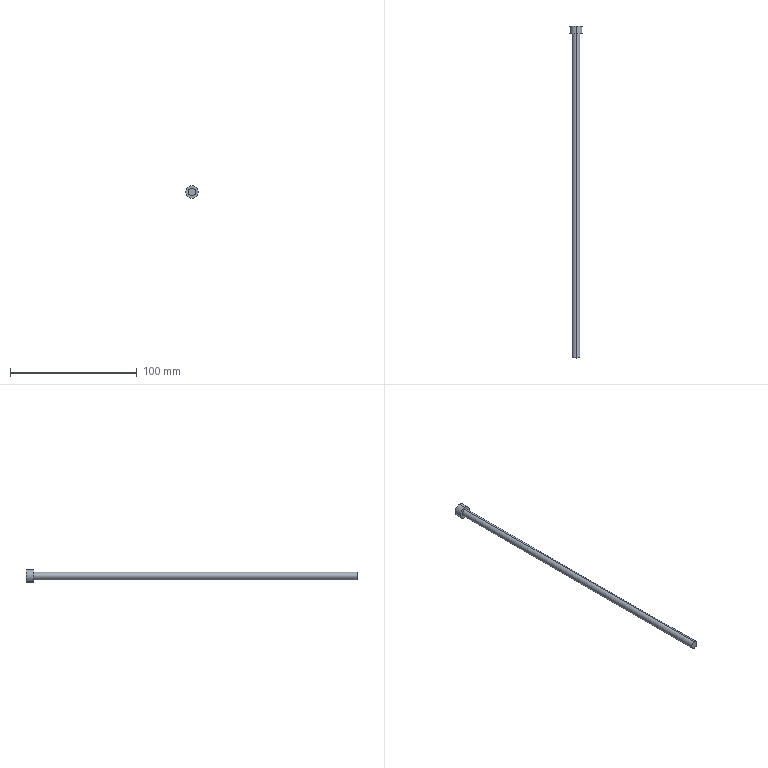Part | STEP file | 1 solid | 7 faces | box 10 x 262.36 x 10 mm | volume 7720 mm3 | cylinder 4 | plane 3 | commonest cylinder face diameters 6 x2 10 x2
STEP:
#1=CARTESIAN_POINT('',(0.,0.,0.));
#2=DIRECTION('',(0.,0.,1.));
#3=DIRECTION('',(1.,0.,0.));
#4=AXIS2_PLACEMENT_3D('',#1,#2,#3);
#5=CARTESIAN_POINT('',(-135.864,290.5,51.072));
#6=VERTEX_POINT('',#5);
#7=CARTESIAN_POINT('',(-135.864,290.5,61.072));
#8=VERTEX_POINT('',#7);
#9=CARTESIAN_POINT('',(-135.864,290.5,56.072));
#10=DIRECTION('',(0.,-1.,0.));
#11=DIRECTION('',(0.,0.,-1.));
#12=AXIS2_PLACEMENT_3D('',#9,#10,#11);
#13=CIRCLE('',#12,5.);
#14=CARTESIAN_POINT('',(-135.864,290.5,56.072));
#15=DIRECTION('',(0.,-1.,0.));
#16=DIRECTION('',(0.,0.,-1.));
#17=AXIS2_PLACEMENT_3D('',#14,#15,#16);
#18=CYLINDRICAL_SURFACE('',#17,5.);
#19=CARTESIAN_POINT('',(0.,0.));
#20=DIRECTION('',(1.,0.));
#21=VECTOR('',#20,1.);
#22=LINE('',#19,#21);
#23=(GEOMETRIC_REPRESENTATION_CONTEXT(2)PARAMETRIC_REPRESENTATION_CONTEXT()REPRESENTATION_CONTEXT('',''));
#24=DEFINITIONAL_REPRESENTATION('',(#22),#23);
#25=PCURVE('',#18,#24);
#26=CARTESIAN_POINT('',(-72.862,290.5,110.196));
#27=DIRECTION('',(0.,-1.,0.));
#28=DIRECTION('',(0.,0.,-1.));
#29=AXIS2_PLACEMENT_3D('',#26,#27,#28);
#30=PLANE('',#29);
#31=CARTESIAN_POINT('',(54.123,-63.002));
#32=DIRECTION('',(1.,0.));
#33=AXIS2_PLACEMENT_2D('',#31,#32);
#34=CIRCLE('',#33,5.);
#35=(GEOMETRIC_REPRESENTATION_CONTEXT(2)PARAMETRIC_REPRESENTATION_CONTEXT()REPRESENTATION_CONTEXT('',''));
#36=DEFINITIONAL_REPRESENTATION('',(#34),#35);
#37=PCURVE('',#30,#36);
#38=SURFACE_CURVE('',#13,(#25,#37),.PCURVE_S1.);
#39=EDGE_CURVE('',#6,#8,#38,.T.);
#40=ORIENTED_EDGE('',*,*,#39,.T.);
#41=CARTESIAN_POINT('',(-135.864,284.5,61.072));
#42=VERTEX_POINT('',#41);
#43=CARTESIAN_POINT('',(-135.864,290.5,61.072));
#44=DIRECTION('',(0.,-1.,0.));
#45=VECTOR('',#44,1.);
#46=LINE('',#43,#45);
#47=CARTESIAN_POINT('',(3.142,0.));
#48=DIRECTION('',(0.,1.));
#49=VECTOR('',#48,1.);
#50=LINE('',#47,#49);
#51=(GEOMETRIC_REPRESENTATION_CONTEXT(2)PARAMETRIC_REPRESENTATION_CONTEXT()REPRESENTATION_CONTEXT('',''));
#52=DEFINITIONAL_REPRESENTATION('',(#50),#51);
#53=PCURVE('',#18,#52);
#54=CARTESIAN_POINT('',(-135.864,290.5,56.072));
#55=DIRECTION('',(0.,-1.,0.));
#56=DIRECTION('',(0.,0.,-1.));
#57=AXIS2_PLACEMENT_3D('',#54,#55,#56);
#58=CYLINDRICAL_SURFACE('',#57,5.);
#59=CARTESIAN_POINT('',(3.142,0.));
#60=DIRECTION('',(0.,1.));
#61=VECTOR('',#60,1.);
#62=LINE('',#59,#61);
#63=(GEOMETRIC_REPRESENTATION_CONTEXT(2)PARAMETRIC_REPRESENTATION_CONTEXT()REPRESENTATION_CONTEXT('',''));
#64=DEFINITIONAL_REPRESENTATION('',(#62),#63);
#65=PCURVE('',#58,#64);
#66=SURFACE_CURVE('',#46,(#53,#65),.PCURVE_S1.);
#67=EDGE_CURVE('',#8,#42,#66,.T.);
#68=ORIENTED_EDGE('',*,*,#67,.T.);
#69=CARTESIAN_POINT('',(-135.864,284.5,51.072));
#70=VERTEX_POINT('',#69);
#71=CARTESIAN_POINT('',(-135.864,284.5,56.072));
#72=DIRECTION('',(0.,1.,0.));
#73=DIRECTION('',(0.,0.,1.));
#74=AXIS2_PLACEMENT_3D('',#71,#72,#73);
#75=CIRCLE('',#74,5.);
#76=CARTESIAN_POINT('',(3.142,6.));
#77=DIRECTION('',(-1.,0.));
#78=VECTOR('',#77,1.);
#79=LINE('',#76,#78);
#80=(GEOMETRIC_REPRESENTATION_CONTEXT(2)PARAMETRIC_REPRESENTATION_CONTEXT()REPRESENTATION_CONTEXT('',''));
#81=DEFINITIONAL_REPRESENTATION('',(#79),#80);
#82=PCURVE('',#18,#81);
#83=CARTESIAN_POINT('',(-135.864,284.5,56.072));
#84=DIRECTION('',(0.,-1.,0.));
#85=DIRECTION('',(0.,0.,-1.));
#86=AXIS2_PLACEMENT_3D('',#83,#84,#85);
#87=PLANE('',#86);
#88=CARTESIAN_POINT('',(-5.,0.));
#89=CARTESIAN_POINT('',(-5.,8.66));
#90=CARTESIAN_POINT('',(2.5,4.33));
#91=CARTESIAN_POINT('',(10.,0.));
#92=CARTESIAN_POINT('',(2.5,-4.33));
#93=CARTESIAN_POINT('',(-5.,-8.66));
#94=CARTESIAN_POINT('',(-5.,0.));
#95=(BOUNDED_CURVE()B_SPLINE_CURVE(2,(#88,#89,#90,#91,#92,#93,#94),.UNSPECIFIED.,.T.,.F.)B_SPLINE_CURVE_WITH_KNOTS((1,2,2,2,2,1),(-2.094,0.,2.094,4.189,6.283,8.378),.UNSPECIFIED.)CURVE()GEOMETRIC_REPRESENTATION_ITEM()RATIONAL_B_SPLINE_CURVE((1.,0.5,1.,0.5,1.,0.5,1.))REPRESENTATION_ITEM(''));
#96=(GEOMETRIC_REPRESENTATION_CONTEXT(2)PARAMETRIC_REPRESENTATION_CONTEXT()REPRESENTATION_CONTEXT('',''));
#97=DEFINITIONAL_REPRESENTATION('',(#95),#96);
#98=PCURVE('',#87,#97);
#99=SURFACE_CURVE('',#75,(#82,#98),.PCURVE_S1.);
#100=EDGE_CURVE('',#42,#70,#99,.T.);
#101=ORIENTED_EDGE('',*,*,#100,.T.);
#102=CARTESIAN_POINT('',(-135.864,290.5,51.072));
#103=DIRECTION('',(0.,-1.,0.));
#104=VECTOR('',#103,1.);
#105=LINE('',#102,#104);
#106=CARTESIAN_POINT('',(0.,0.));
#107=DIRECTION('',(0.,1.));
#108=VECTOR('',#107,1.);
#109=LINE('',#106,#108);
#110=(GEOMETRIC_REPRESENTATION_CONTEXT(2)PARAMETRIC_REPRESENTATION_CONTEXT()REPRESENTATION_CONTEXT('',''));
#111=DEFINITIONAL_REPRESENTATION('',(#109),#110);
#112=PCURVE('',#18,#111);
#113=CARTESIAN_POINT('',(6.283,0.));
#114=DIRECTION('',(0.,1.));
#115=VECTOR('',#114,1.);
#116=LINE('',#113,#115);
#117=(GEOMETRIC_REPRESENTATION_CONTEXT(2)PARAMETRIC_REPRESENTATION_CONTEXT()REPRESENTATION_CONTEXT('',''));
#118=DEFINITIONAL_REPRESENTATION('',(#116),#117);
#119=PCURVE('',#58,#118);
#120=SURFACE_CURVE('',#105,(#112,#119),.PCURVE_S1.);
#121=EDGE_CURVE('',#6,#70,#120,.T.);
#122=ORIENTED_EDGE('',*,*,#121,.F.);
#123=EDGE_LOOP('',(#40,#68,#101,#122));
#124=FACE_BOUND('',#123,.T.);
#125=ADVANCED_FACE('',(#124),#18,.T.);
#126=CARTESIAN_POINT('',(-135.864,284.5,59.072));
#127=VERTEX_POINT('',#126);
#128=CARTESIAN_POINT('',(-135.864,284.5,53.072));
#129=VERTEX_POINT('',#128);
#130=CARTESIAN_POINT('',(-135.864,284.5,56.072));
#131=DIRECTION('',(0.,1.,0.));
#132=DIRECTION('',(0.,0.,-1.));
#133=AXIS2_PLACEMENT_3D('',#130,#131,#132);
#134=CIRCLE('',#133,3.);
#135=CARTESIAN_POINT('',(-135.864,220.5,56.072));
#136=DIRECTION('',(0.,-1.,0.));
#137=DIRECTION('',(0.,0.,-1.));
#138=AXIS2_PLACEMENT_3D('',#135,#136,#137);
#139=CYLINDRICAL_SURFACE('',#138,3.);
#140=CARTESIAN_POINT('',(6.283,-64.));
#141=DIRECTION('',(-1.,0.));
#142=VECTOR('',#141,1.);
#143=LINE('',#140,#142);
#144=(GEOMETRIC_REPRESENTATION_CONTEXT(2)PARAMETRIC_REPRESENTATION_CONTEXT()REPRESENTATION_CONTEXT('',''));
#145=DEFINITIONAL_REPRESENTATION('',(#143),#144);
#146=PCURVE('',#139,#145);
#147=CARTESIAN_POINT('',(3.,0.));
#148=CARTESIAN_POINT('',(3.,-5.196));
#149=CARTESIAN_POINT('',(-1.5,-2.598));
#150=CARTESIAN_POINT('',(-6.,0.));
#151=CARTESIAN_POINT('',(-1.5,2.598));
#152=CARTESIAN_POINT('',(3.,5.196));
#153=CARTESIAN_POINT('',(3.,0.));
#154=(BOUNDED_CURVE()B_SPLINE_CURVE(2,(#147,#148,#149,#150,#151,#152,#153),.UNSPECIFIED.,.T.,.F.)B_SPLINE_CURVE_WITH_KNOTS((1,2,2,2,2,1),(-2.094,0.,2.094,4.189,6.283,8.378),.UNSPECIFIED.)CURVE()GEOMETRIC_REPRESENTATION_ITEM()RATIONAL_B_SPLINE_CURVE((1.,0.5,1.,0.5,1.,0.5,1.))REPRESENTATION_ITEM(''));
#155=(GEOMETRIC_REPRESENTATION_CONTEXT(2)PARAMETRIC_REPRESENTATION_CONTEXT()REPRESENTATION_CONTEXT('',''));
#156=DEFINITIONAL_REPRESENTATION('',(#154),#155);
#157=PCURVE('',#87,#156);
#158=SURFACE_CURVE('',#134,(#146,#157),.PCURVE_S1.);
#159=EDGE_CURVE('',#127,#129,#158,.T.);
#160=ORIENTED_EDGE('',*,*,#159,.F.);
#161=CARTESIAN_POINT('',(-135.864,28.14,59.072));
#162=VERTEX_POINT('',#161);
#163=CARTESIAN_POINT('',(-135.864,220.5,59.072));
#164=DIRECTION('',(0.,-1.,0.));
#165=VECTOR('',#164,1.);
#166=LINE('',#163,#165);
#167=CARTESIAN_POINT('',(3.142,0.));
#168=DIRECTION('',(0.,1.));
#169=VECTOR('',#168,1.);
#170=LINE('',#167,#169);
#171=(GEOMETRIC_REPRESENTATION_CONTEXT(2)PARAMETRIC_REPRESENTATION_CONTEXT()REPRESENTATION_CONTEXT('',''));
#172=DEFINITIONAL_REPRESENTATION('',(#170),#171);
#173=PCURVE('',#139,#172);
#174=CARTESIAN_POINT('',(-135.864,220.5,56.072));
#175=DIRECTION('',(0.,-1.,0.));
#176=DIRECTION('',(0.,0.,-1.));
#177=AXIS2_PLACEMENT_3D('',#174,#175,#176);
#178=CYLINDRICAL_SURFACE('',#177,3.);
#179=CARTESIAN_POINT('',(3.142,0.));
#180=DIRECTION('',(0.,1.));
#181=VECTOR('',#180,1.);
#182=LINE('',#179,#181);
#183=(GEOMETRIC_REPRESENTATION_CONTEXT(2)PARAMETRIC_REPRESENTATION_CONTEXT()REPRESENTATION_CONTEXT('',''));
#184=DEFINITIONAL_REPRESENTATION('',(#182),#183);
#185=PCURVE('',#178,#184);
#186=SURFACE_CURVE('',#166,(#173,#185),.PCURVE_S1.);
#187=EDGE_CURVE('',#127,#162,#186,.T.);
#188=ORIENTED_EDGE('',*,*,#187,.T.);
#189=CARTESIAN_POINT('',(-135.864,28.14,53.072));
#190=VERTEX_POINT('',#189);
#191=CARTESIAN_POINT('',(-135.864,28.14,56.072));
#192=DIRECTION('',(0.,1.,0.));
#193=DIRECTION('',(0.,0.,-1.));
#194=AXIS2_PLACEMENT_3D('',#191,#192,#193);
#195=CIRCLE('',#194,3.);
#196=CARTESIAN_POINT('',(6.283,192.36));
#197=DIRECTION('',(-1.,0.));
#198=VECTOR('',#197,1.);
#199=LINE('',#196,#198);
#200=(GEOMETRIC_REPRESENTATION_CONTEXT(2)PARAMETRIC_REPRESENTATION_CONTEXT()REPRESENTATION_CONTEXT('',''));
#201=DEFINITIONAL_REPRESENTATION('',(#199),#200);
#202=PCURVE('',#139,#201);
#203=CARTESIAN_POINT('',(-72.862,28.14,-91.563));
#204=DIRECTION('',(0.,-1.,0.));
#205=DIRECTION('',(0.,0.,-1.));
#206=AXIS2_PLACEMENT_3D('',#203,#204,#205);
#207=PLANE('',#206);
#208=CARTESIAN_POINT('',(-144.636,-63.002));
#209=CARTESIAN_POINT('',(-144.636,-68.198));
#210=CARTESIAN_POINT('',(-149.136,-65.6));
#211=CARTESIAN_POINT('',(-153.636,-63.002));
#212=CARTESIAN_POINT('',(-149.136,-60.404));
#213=CARTESIAN_POINT('',(-144.636,-57.806));
#214=CARTESIAN_POINT('',(-144.636,-63.002));
#215=(BOUNDED_CURVE()B_SPLINE_CURVE(2,(#208,#209,#210,#211,#212,#213,#214),.UNSPECIFIED.,.T.,.F.)B_SPLINE_CURVE_WITH_KNOTS((1,2,2,2,2,1),(-2.094,0.,2.094,4.189,6.283,8.378),.UNSPECIFIED.)CURVE()GEOMETRIC_REPRESENTATION_ITEM()RATIONAL_B_SPLINE_CURVE((1.,0.5,1.,0.5,1.,0.5,1.))REPRESENTATION_ITEM(''));
#216=(GEOMETRIC_REPRESENTATION_CONTEXT(2)PARAMETRIC_REPRESENTATION_CONTEXT()REPRESENTATION_CONTEXT('',''));
#217=DEFINITIONAL_REPRESENTATION('',(#215),#216);
#218=PCURVE('',#207,#217);
#219=SURFACE_CURVE('',#195,(#202,#218),.PCURVE_S1.);
#220=EDGE_CURVE('',#162,#190,#219,.T.);
#221=ORIENTED_EDGE('',*,*,#220,.T.);
#222=CARTESIAN_POINT('',(-135.864,220.5,53.072));
#223=DIRECTION('',(0.,-1.,0.));
#224=VECTOR('',#223,1.);
#225=LINE('',#222,#224);
#226=CARTESIAN_POINT('',(0.,0.));
#227=DIRECTION('',(0.,1.));
#228=VECTOR('',#227,1.);
#229=LINE('',#226,#228);
#230=(GEOMETRIC_REPRESENTATION_CONTEXT(2)PARAMETRIC_REPRESENTATION_CONTEXT()REPRESENTATION_CONTEXT('',''));
#231=DEFINITIONAL_REPRESENTATION('',(#229),#230);
#232=PCURVE('',#139,#231);
#233=CARTESIAN_POINT('',(6.283,0.));
#234=DIRECTION('',(0.,1.));
#235=VECTOR('',#234,1.);
#236=LINE('',#233,#235);
#237=(GEOMETRIC_REPRESENTATION_CONTEXT(2)PARAMETRIC_REPRESENTATION_CONTEXT()REPRESENTATION_CONTEXT('',''));
#238=DEFINITIONAL_REPRESENTATION('',(#236),#237);
#239=PCURVE('',#178,#238);
#240=SURFACE_CURVE('',#225,(#232,#239),.PCURVE_S1.);
#241=EDGE_CURVE('',#129,#190,#240,.T.);
#242=ORIENTED_EDGE('',*,*,#241,.F.);
#243=EDGE_LOOP('',(#160,#188,#221,#242));
#244=FACE_BOUND('',#243,.T.);
#245=ADVANCED_FACE('',(#244),#139,.T.);
#246=ORIENTED_EDGE('',*,*,#187,.F.);
#247=CARTESIAN_POINT('',(-135.864,284.5,56.072));
#248=DIRECTION('',(0.,1.,0.));
#249=DIRECTION('',(0.,0.,-1.));
#250=AXIS2_PLACEMENT_3D('',#247,#248,#249);
#251=CIRCLE('',#250,3.);
#252=CARTESIAN_POINT('',(6.283,-64.));
#253=DIRECTION('',(-1.,0.));
#254=VECTOR('',#253,1.);
#255=LINE('',#252,#254);
#256=(GEOMETRIC_REPRESENTATION_CONTEXT(2)PARAMETRIC_REPRESENTATION_CONTEXT()REPRESENTATION_CONTEXT('',''));
#257=DEFINITIONAL_REPRESENTATION('',(#255),#256);
#258=PCURVE('',#178,#257);
#259=CARTESIAN_POINT('',(3.,0.));
#260=CARTESIAN_POINT('',(3.,-5.196));
#261=CARTESIAN_POINT('',(-1.5,-2.598));
#262=CARTESIAN_POINT('',(-6.,0.));
#263=CARTESIAN_POINT('',(-1.5,2.598));
#264=CARTESIAN_POINT('',(3.,5.196));
#265=CARTESIAN_POINT('',(3.,0.));
#266=(BOUNDED_CURVE()B_SPLINE_CURVE(2,(#259,#260,#261,#262,#263,#264,#265),.UNSPECIFIED.,.T.,.F.)B_SPLINE_CURVE_WITH_KNOTS((1,2,2,2,2,1),(-2.094,0.,2.094,4.189,6.283,8.378),.UNSPECIFIED.)CURVE()GEOMETRIC_REPRESENTATION_ITEM()RATIONAL_B_SPLINE_CURVE((1.,0.5,1.,0.5,1.,0.5,1.))REPRESENTATION_ITEM(''));
#267=(GEOMETRIC_REPRESENTATION_CONTEXT(2)PARAMETRIC_REPRESENTATION_CONTEXT()REPRESENTATION_CONTEXT('',''));
#268=DEFINITIONAL_REPRESENTATION('',(#266),#267);
#269=PCURVE('',#87,#268);
#270=SURFACE_CURVE('',#251,(#258,#269),.PCURVE_S1.);
#271=EDGE_CURVE('',#129,#127,#270,.T.);
#272=ORIENTED_EDGE('',*,*,#271,.F.);
#273=ORIENTED_EDGE('',*,*,#241,.T.);
#274=CARTESIAN_POINT('',(-135.864,28.14,56.072));
#275=DIRECTION('',(0.,1.,0.));
#276=DIRECTION('',(0.,0.,-1.));
#277=AXIS2_PLACEMENT_3D('',#274,#275,#276);
#278=CIRCLE('',#277,3.);
#279=CARTESIAN_POINT('',(6.283,192.36));
#280=DIRECTION('',(-1.,0.));
#281=VECTOR('',#280,1.);
#282=LINE('',#279,#281);
#283=(GEOMETRIC_REPRESENTATION_CONTEXT(2)PARAMETRIC_REPRESENTATION_CONTEXT()REPRESENTATION_CONTEXT('',''));
#284=DEFINITIONAL_REPRESENTATION('',(#282),#283);
#285=PCURVE('',#178,#284);
#286=CARTESIAN_POINT('',(-144.636,-63.002));
#287=CARTESIAN_POINT('',(-144.636,-68.198));
#288=CARTESIAN_POINT('',(-149.136,-65.6));
#289=CARTESIAN_POINT('',(-153.636,-63.002));
#290=CARTESIAN_POINT('',(-149.136,-60.404));
#291=CARTESIAN_POINT('',(-144.636,-57.806));
#292=CARTESIAN_POINT('',(-144.636,-63.002));
#293=(BOUNDED_CURVE()B_SPLINE_CURVE(2,(#286,#287,#288,#289,#290,#291,#292),.UNSPECIFIED.,.T.,.F.)B_SPLINE_CURVE_WITH_KNOTS((1,2,2,2,2,1),(-2.094,0.,2.094,4.189,6.283,8.378),.UNSPECIFIED.)CURVE()GEOMETRIC_REPRESENTATION_ITEM()RATIONAL_B_SPLINE_CURVE((1.,0.5,1.,0.5,1.,0.5,1.))REPRESENTATION_ITEM(''));
#294=(GEOMETRIC_REPRESENTATION_CONTEXT(2)PARAMETRIC_REPRESENTATION_CONTEXT()REPRESENTATION_CONTEXT('',''));
#295=DEFINITIONAL_REPRESENTATION('',(#293),#294);
#296=PCURVE('',#207,#295);
#297=SURFACE_CURVE('',#278,(#285,#296),.PCURVE_S1.);
#298=EDGE_CURVE('',#190,#162,#297,.T.);
#299=ORIENTED_EDGE('',*,*,#298,.T.);
#300=EDGE_LOOP('',(#246,#272,#273,#299));
#301=FACE_BOUND('',#300,.T.);
#302=ADVANCED_FACE('',(#301),#178,.T.);
#303=ORIENTED_EDGE('',*,*,#298,.F.);
#304=ORIENTED_EDGE('',*,*,#220,.F.);
#305=EDGE_LOOP('',(#303,#304));
#306=FACE_BOUND('',#305,.T.);
#307=ADVANCED_FACE('',(#306),#207,.T.);
#308=ORIENTED_EDGE('',*,*,#271,.T.);
#309=ORIENTED_EDGE('',*,*,#159,.T.);
#310=EDGE_LOOP('',(#308,#309));
#311=FACE_BOUND('',#310,.T.);
#312=CARTESIAN_POINT('',(-135.864,284.5,56.072));
#313=DIRECTION('',(0.,1.,0.));
#314=DIRECTION('',(0.,0.,1.));
#315=AXIS2_PLACEMENT_3D('',#312,#313,#314);
#316=CIRCLE('',#315,5.);
#317=CARTESIAN_POINT('',(-5.,0.));
#318=CARTESIAN_POINT('',(-5.,8.66));
#319=CARTESIAN_POINT('',(2.5,4.33));
#320=CARTESIAN_POINT('',(10.,0.));
#321=CARTESIAN_POINT('',(2.5,-4.33));
#322=CARTESIAN_POINT('',(-5.,-8.66));
#323=CARTESIAN_POINT('',(-5.,0.));
#324=(BOUNDED_CURVE()B_SPLINE_CURVE(2,(#317,#318,#319,#320,#321,#322,#323),.UNSPECIFIED.,.T.,.F.)B_SPLINE_CURVE_WITH_KNOTS((1,2,2,2,2,1),(-2.094,0.,2.094,4.189,6.283,8.378),.UNSPECIFIED.)CURVE()GEOMETRIC_REPRESENTATION_ITEM()RATIONAL_B_SPLINE_CURVE((1.,0.5,1.,0.5,1.,0.5,1.))REPRESENTATION_ITEM(''));
#325=(GEOMETRIC_REPRESENTATION_CONTEXT(2)PARAMETRIC_REPRESENTATION_CONTEXT()REPRESENTATION_CONTEXT('',''));
#326=DEFINITIONAL_REPRESENTATION('',(#324),#325);
#327=PCURVE('',#87,#326);
#328=CARTESIAN_POINT('',(9.425,6.));
#329=DIRECTION('',(-1.,0.));
#330=VECTOR('',#329,1.);
#331=LINE('',#328,#330);
#332=(GEOMETRIC_REPRESENTATION_CONTEXT(2)PARAMETRIC_REPRESENTATION_CONTEXT()REPRESENTATION_CONTEXT('',''));
#333=DEFINITIONAL_REPRESENTATION('',(#331),#332);
#334=PCURVE('',#58,#333);
#335=SURFACE_CURVE('',#316,(#327,#334),.PCURVE_S1.);
#336=EDGE_CURVE('',#70,#42,#335,.T.);
#337=ORIENTED_EDGE('',*,*,#336,.F.);
#338=ORIENTED_EDGE('',*,*,#100,.F.);
#339=EDGE_LOOP('',(#337,#338));
#340=FACE_BOUND('',#339,.T.);
#341=ADVANCED_FACE('',(#311,#340),#87,.T.);
#342=ORIENTED_EDGE('',*,*,#67,.F.);
#343=CARTESIAN_POINT('',(-135.864,290.5,56.072));
#344=DIRECTION('',(0.,-1.,0.));
#345=DIRECTION('',(0.,0.,-1.));
#346=AXIS2_PLACEMENT_3D('',#343,#344,#345);
#347=CIRCLE('',#346,5.);
#348=CARTESIAN_POINT('',(0.,0.));
#349=DIRECTION('',(1.,0.));
#350=VECTOR('',#349,1.);
#351=LINE('',#348,#350);
#352=(GEOMETRIC_REPRESENTATION_CONTEXT(2)PARAMETRIC_REPRESENTATION_CONTEXT()REPRESENTATION_CONTEXT('',''));
#353=DEFINITIONAL_REPRESENTATION('',(#351),#352);
#354=PCURVE('',#58,#353);
#355=CARTESIAN_POINT('',(54.123,-63.002));
#356=DIRECTION('',(1.,0.));
#357=AXIS2_PLACEMENT_2D('',#355,#356);
#358=CIRCLE('',#357,5.);
#359=(GEOMETRIC_REPRESENTATION_CONTEXT(2)PARAMETRIC_REPRESENTATION_CONTEXT()REPRESENTATION_CONTEXT('',''));
#360=DEFINITIONAL_REPRESENTATION('',(#358),#359);
#361=PCURVE('',#30,#360);
#362=SURFACE_CURVE('',#347,(#354,#361),.PCURVE_S1.);
#363=EDGE_CURVE('',#8,#6,#362,.T.);
#364=ORIENTED_EDGE('',*,*,#363,.T.);
#365=ORIENTED_EDGE('',*,*,#121,.T.);
#366=ORIENTED_EDGE('',*,*,#336,.T.);
#367=EDGE_LOOP('',(#342,#364,#365,#366));
#368=FACE_BOUND('',#367,.T.);
#369=ADVANCED_FACE('',(#368),#58,.T.);
#370=ORIENTED_EDGE('',*,*,#39,.F.);
#371=ORIENTED_EDGE('',*,*,#363,.F.);
#372=EDGE_LOOP('',(#370,#371));
#373=FACE_BOUND('',#372,.T.);
#374=ADVANCED_FACE('',(#373),#30,.F.);
#375=CLOSED_SHELL('',(#125,#245,#302,#307,#341,#369,#374));
#376=MANIFOLD_SOLID_BREP('',#375);
#377=(LENGTH_UNIT()NAMED_UNIT(*)SI_UNIT(.MILLI.,.METRE.));
#378=UNCERTAINTY_MEASURE_WITH_UNIT(LENGTH_MEASURE(0.0000001),#377,'','');
#379=(NAMED_UNIT(*)PLANE_ANGLE_UNIT()SI_UNIT($,.RADIAN.));
#380=(NAMED_UNIT(*)SI_UNIT($,.STERADIAN.)SOLID_ANGLE_UNIT());
#381=(GEOMETRIC_REPRESENTATION_CONTEXT(3)GLOBAL_UNCERTAINTY_ASSIGNED_CONTEXT((#378))GLOBAL_UNIT_ASSIGNED_CONTEXT((#377,#379,#380))REPRESENTATION_CONTEXT('',''));
#382=ADVANCED_BREP_SHAPE_REPRESENTATION('',(#4,#376),#381);